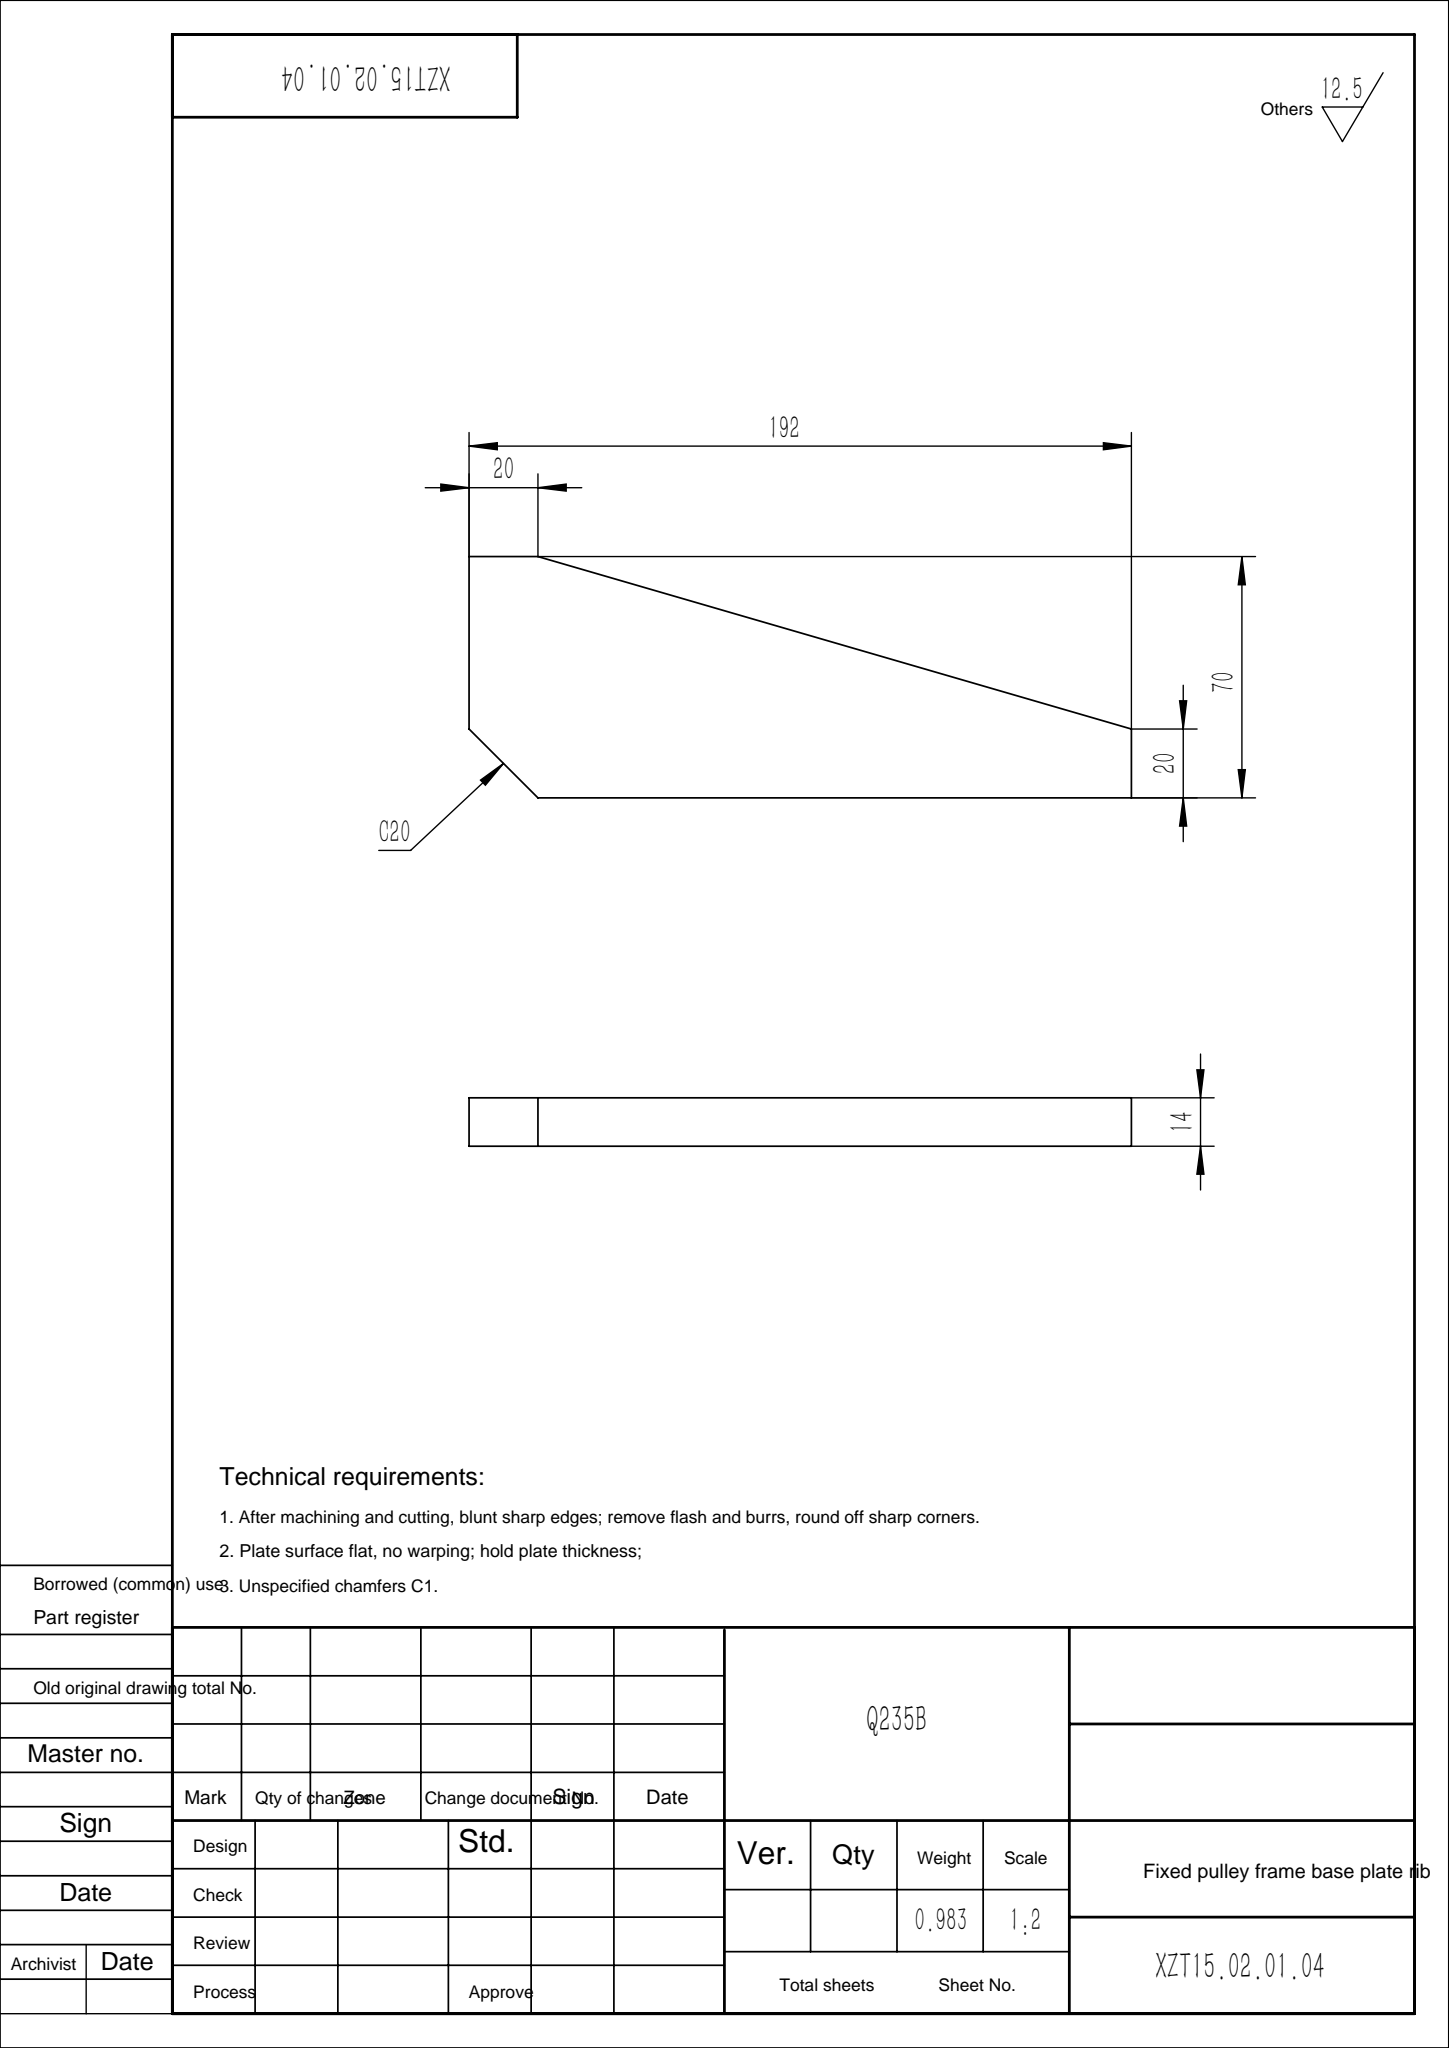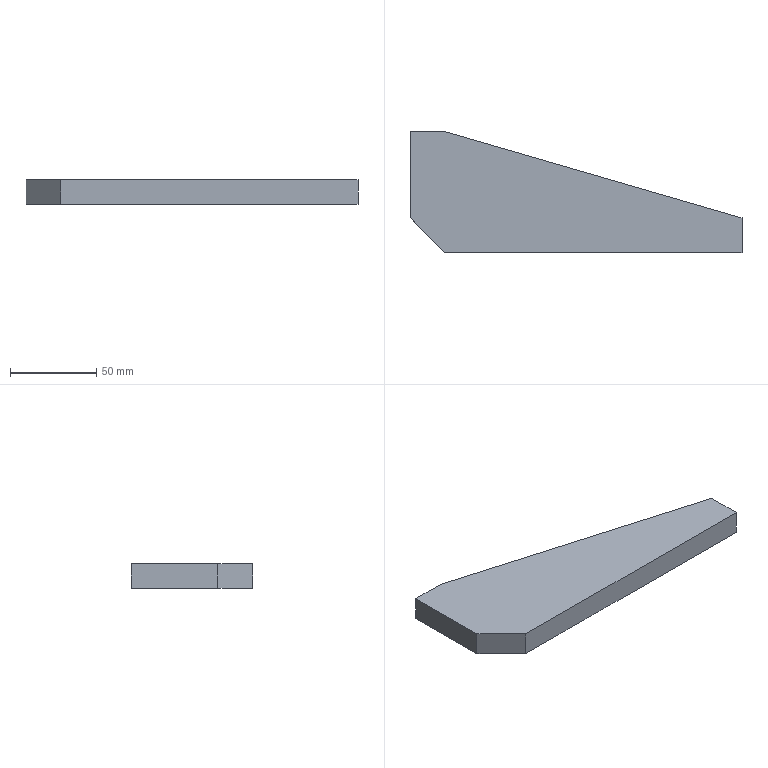Part | SolidWorks | features Chamfer 1, Extrusion 1 | 1 solid | 8 faces | box 192 x 70 x 14 mm | volume 125160 mm3 | plane 8
STEP:
#1=CARTESIAN_POINT('',(0.,70.,-7.));
#2=VERTEX_POINT('',#1);
#3=CARTESIAN_POINT('',(0.,20.,-7.));
#4=VERTEX_POINT('',#3);
#5=CARTESIAN_POINT('',(0.,70.,-7.));
#6=DIRECTION('',(0.,-1.,0.));
#7=VECTOR('',#6,1000.);
#8=LINE('',#5,#7);
#9=EDGE_CURVE('',#2,#4,#8,.T.);
#10=ORIENTED_EDGE('',*,*,#9,.T.);
#11=CARTESIAN_POINT('',(0.,20.,7.));
#12=VERTEX_POINT('',#11);
#13=CARTESIAN_POINT('',(0.,20.,7.));
#14=DIRECTION('',(0.,0.,1.));
#15=VECTOR('',#14,1000.);
#16=LINE('',#13,#15);
#17=EDGE_CURVE('',#4,#12,#16,.T.);
#18=ORIENTED_EDGE('',*,*,#17,.T.);
#19=CARTESIAN_POINT('',(0.,70.,7.));
#20=VERTEX_POINT('',#19);
#21=CARTESIAN_POINT('',(0.,70.,7.));
#22=DIRECTION('',(0.,-1.,0.));
#23=VECTOR('',#22,1000.);
#24=LINE('',#21,#23);
#25=EDGE_CURVE('',#20,#12,#24,.T.);
#26=ORIENTED_EDGE('',*,*,#25,.F.);
#27=CARTESIAN_POINT('',(0.,70.,7.));
#28=DIRECTION('',(0.,0.,-1.));
#29=VECTOR('',#28,1000.);
#30=LINE('',#27,#29);
#31=EDGE_CURVE('',#20,#2,#30,.T.);
#32=ORIENTED_EDGE('',*,*,#31,.T.);
#33=EDGE_LOOP('',(#10,#18,#26,#32));
#34=FACE_OUTER_BOUND('',#33,.T.);
#35=CARTESIAN_POINT('',(0.,70.,7.));
#36=DIRECTION('',(1.,0.,0.));
#37=DIRECTION('',(0.,1.,0.));
#38=AXIS2_PLACEMENT_3D('',#35,#36,#37);
#39=PLANE('',#38);
#40=ADVANCED_FACE('',(#34),#39,.F.);
#41=CARTESIAN_POINT('',(20.,0.,7.));
#42=VERTEX_POINT('',#41);
#43=CARTESIAN_POINT('',(192.,0.,7.));
#44=VERTEX_POINT('',#43);
#45=CARTESIAN_POINT('',(0.,0.,7.));
#46=DIRECTION('',(1.,0.,0.));
#47=VECTOR('',#46,1000.);
#48=LINE('',#45,#47);
#49=EDGE_CURVE('',#42,#44,#48,.T.);
#50=ORIENTED_EDGE('',*,*,#49,.F.);
#51=CARTESIAN_POINT('',(20.,0.,-7.));
#52=VERTEX_POINT('',#51);
#53=CARTESIAN_POINT('',(20.,0.,7.));
#54=DIRECTION('',(0.,0.,-1.));
#55=VECTOR('',#54,1000.);
#56=LINE('',#53,#55);
#57=EDGE_CURVE('',#42,#52,#56,.T.);
#58=ORIENTED_EDGE('',*,*,#57,.T.);
#59=CARTESIAN_POINT('',(192.,0.,-7.));
#60=VERTEX_POINT('',#59);
#61=CARTESIAN_POINT('',(0.,0.,-7.));
#62=DIRECTION('',(1.,0.,0.));
#63=VECTOR('',#62,1000.);
#64=LINE('',#61,#63);
#65=EDGE_CURVE('',#52,#60,#64,.T.);
#66=ORIENTED_EDGE('',*,*,#65,.T.);
#67=CARTESIAN_POINT('',(192.,0.,7.));
#68=DIRECTION('',(0.,0.,-1.));
#69=VECTOR('',#68,1000.);
#70=LINE('',#67,#69);
#71=EDGE_CURVE('',#44,#60,#70,.T.);
#72=ORIENTED_EDGE('',*,*,#71,.F.);
#73=EDGE_LOOP('',(#50,#58,#66,#72));
#74=FACE_OUTER_BOUND('',#73,.T.);
#75=CARTESIAN_POINT('',(0.,0.,7.));
#76=DIRECTION('',(0.,1.,0.));
#77=DIRECTION('',(0.,0.,1.));
#78=AXIS2_PLACEMENT_3D('',#75,#76,#77);
#79=PLANE('',#78);
#80=ADVANCED_FACE('',(#74),#79,.F.);
#81=CARTESIAN_POINT('',(192.,20.,-7.));
#82=VERTEX_POINT('',#81);
#83=CARTESIAN_POINT('',(192.,0.,-7.));
#84=DIRECTION('',(0.,1.,0.));
#85=VECTOR('',#84,1000.);
#86=LINE('',#83,#85);
#87=EDGE_CURVE('',#60,#82,#86,.T.);
#88=ORIENTED_EDGE('',*,*,#87,.T.);
#89=CARTESIAN_POINT('',(192.,20.,7.));
#90=VERTEX_POINT('',#89);
#91=CARTESIAN_POINT('',(192.,20.,7.));
#92=DIRECTION('',(0.,0.,-1.));
#93=VECTOR('',#92,1000.);
#94=LINE('',#91,#93);
#95=EDGE_CURVE('',#90,#82,#94,.T.);
#96=ORIENTED_EDGE('',*,*,#95,.F.);
#97=CARTESIAN_POINT('',(192.,0.,7.));
#98=DIRECTION('',(0.,1.,0.));
#99=VECTOR('',#98,1000.);
#100=LINE('',#97,#99);
#101=EDGE_CURVE('',#44,#90,#100,.T.);
#102=ORIENTED_EDGE('',*,*,#101,.F.);
#103=ORIENTED_EDGE('',*,*,#71,.T.);
#104=EDGE_LOOP('',(#88,#96,#102,#103));
#105=FACE_OUTER_BOUND('',#104,.T.);
#106=CARTESIAN_POINT('',(192.,0.,7.));
#107=DIRECTION('',(-1.,0.,0.));
#108=DIRECTION('',(0.,0.,1.));
#109=AXIS2_PLACEMENT_3D('',#106,#107,#108);
#110=PLANE('',#109);
#111=ADVANCED_FACE('',(#105),#110,.F.);
#112=CARTESIAN_POINT('',(20.,70.,-7.));
#113=VERTEX_POINT('',#112);
#114=CARTESIAN_POINT('',(192.,20.,-7.));
#115=DIRECTION('',(-0.9602,0.2791,0.));
#116=VECTOR('',#115,1000.);
#117=LINE('',#114,#116);
#118=EDGE_CURVE('',#82,#113,#117,.T.);
#119=ORIENTED_EDGE('',*,*,#118,.T.);
#120=CARTESIAN_POINT('',(20.,70.,7.));
#121=VERTEX_POINT('',#120);
#122=CARTESIAN_POINT('',(20.,70.,7.));
#123=DIRECTION('',(0.,0.,-1.));
#124=VECTOR('',#123,1000.);
#125=LINE('',#122,#124);
#126=EDGE_CURVE('',#121,#113,#125,.T.);
#127=ORIENTED_EDGE('',*,*,#126,.F.);
#128=CARTESIAN_POINT('',(192.,20.,7.));
#129=DIRECTION('',(-0.9602,0.2791,0.));
#130=VECTOR('',#129,1000.);
#131=LINE('',#128,#130);
#132=EDGE_CURVE('',#90,#121,#131,.T.);
#133=ORIENTED_EDGE('',*,*,#132,.F.);
#134=ORIENTED_EDGE('',*,*,#95,.T.);
#135=EDGE_LOOP('',(#119,#127,#133,#134));
#136=FACE_OUTER_BOUND('',#135,.T.);
#137=CARTESIAN_POINT('',(192.,20.,7.));
#138=DIRECTION('',(-0.2791,-0.9602,0.));
#139=DIRECTION('',(0.9602,-0.2791,0.));
#140=AXIS2_PLACEMENT_3D('',#137,#138,#139);
#141=PLANE('',#140);
#142=ADVANCED_FACE('',(#136),#141,.F.);
#143=CARTESIAN_POINT('',(20.,70.,-7.));
#144=DIRECTION('',(-1.,0.,0.));
#145=VECTOR('',#144,1000.);
#146=LINE('',#143,#145);
#147=EDGE_CURVE('',#113,#2,#146,.T.);
#148=ORIENTED_EDGE('',*,*,#147,.T.);
#149=ORIENTED_EDGE('',*,*,#31,.F.);
#150=CARTESIAN_POINT('',(20.,70.,7.));
#151=DIRECTION('',(-1.,0.,0.));
#152=VECTOR('',#151,1000.);
#153=LINE('',#150,#152);
#154=EDGE_CURVE('',#121,#20,#153,.T.);
#155=ORIENTED_EDGE('',*,*,#154,.F.);
#156=ORIENTED_EDGE('',*,*,#126,.T.);
#157=EDGE_LOOP('',(#148,#149,#155,#156));
#158=FACE_OUTER_BOUND('',#157,.T.);
#159=CARTESIAN_POINT('',(20.,70.,7.));
#160=DIRECTION('',(0.,-1.,0.));
#161=DIRECTION('',(0.,0.,-1.));
#162=AXIS2_PLACEMENT_3D('',#159,#160,#161);
#163=PLANE('',#162);
#164=ADVANCED_FACE('',(#158),#163,.F.);
#165=ORIENTED_EDGE('',*,*,#25,.T.);
#166=CARTESIAN_POINT('',(10.,10.,7.));
#167=DIRECTION('',(0.7071,-0.7071,0.));
#168=VECTOR('',#167,1000.);
#169=LINE('',#166,#168);
#170=EDGE_CURVE('',#12,#42,#169,.T.);
#171=ORIENTED_EDGE('',*,*,#170,.T.);
#172=ORIENTED_EDGE('',*,*,#49,.T.);
#173=ORIENTED_EDGE('',*,*,#101,.T.);
#174=ORIENTED_EDGE('',*,*,#132,.T.);
#175=ORIENTED_EDGE('',*,*,#154,.T.);
#176=EDGE_LOOP('',(#165,#171,#172,#173,#174,#175));
#177=FACE_OUTER_BOUND('',#176,.T.);
#178=CARTESIAN_POINT('',(0.,0.,7.));
#179=DIRECTION('',(0.,0.,1.));
#180=DIRECTION('',(1.,0.,0.));
#181=AXIS2_PLACEMENT_3D('',#178,#179,#180);
#182=PLANE('',#181);
#183=ADVANCED_FACE('',(#177),#182,.T.);
#184=ORIENTED_EDGE('',*,*,#65,.F.);
#185=CARTESIAN_POINT('',(20.,0.,-7.));
#186=DIRECTION('',(-0.7071,0.7071,0.));
#187=VECTOR('',#186,1000.);
#188=LINE('',#185,#187);
#189=EDGE_CURVE('',#52,#4,#188,.T.);
#190=ORIENTED_EDGE('',*,*,#189,.T.);
#191=ORIENTED_EDGE('',*,*,#9,.F.);
#192=ORIENTED_EDGE('',*,*,#147,.F.);
#193=ORIENTED_EDGE('',*,*,#118,.F.);
#194=ORIENTED_EDGE('',*,*,#87,.F.);
#195=EDGE_LOOP('',(#184,#190,#191,#192,#193,#194));
#196=FACE_OUTER_BOUND('',#195,.T.);
#197=CARTESIAN_POINT('',(0.,0.,-7.));
#198=DIRECTION('',(0.,0.,1.));
#199=DIRECTION('',(1.,0.,0.));
#200=AXIS2_PLACEMENT_3D('',#197,#198,#199);
#201=PLANE('',#200);
#202=ADVANCED_FACE('',(#196),#201,.F.);
#203=ORIENTED_EDGE('',*,*,#170,.F.);
#204=ORIENTED_EDGE('',*,*,#17,.F.);
#205=ORIENTED_EDGE('',*,*,#189,.F.);
#206=ORIENTED_EDGE('',*,*,#57,.F.);
#207=EDGE_LOOP('',(#203,#204,#205,#206));
#208=FACE_OUTER_BOUND('',#207,.T.);
#209=CARTESIAN_POINT('',(20.,0.,7.));
#210=DIRECTION('',(0.7071,0.7071,0.));
#211=DIRECTION('',(0.,0.,-1.));
#212=AXIS2_PLACEMENT_3D('',#209,#210,#211);
#213=PLANE('',#212);
#214=ADVANCED_FACE('',(#208),#213,.F.);
#215=CLOSED_SHELL('',(#40,#80,#111,#142,#164,#183,#202,#214));
#216=MANIFOLD_SOLID_BREP('',#215);
#217=CARTESIAN_POINT('',(0.,0.,0.));
#218=DIRECTION('',(0.,0.,1.));
#219=DIRECTION('',(1.,0.,0.));
#220=AXIS2_PLACEMENT_3D('',#217,#218,#219);
#221=(LENGTH_UNIT()NAMED_UNIT(*)SI_UNIT(.MILLI.,.METRE.));
#222=UNCERTAINTY_MEASURE_WITH_UNIT(LENGTH_MEASURE(0.00001),#221,'','');
#223=(NAMED_UNIT(*)PLANE_ANGLE_UNIT()SI_UNIT($,.RADIAN.));
#224=(NAMED_UNIT(*)SI_UNIT($,.STERADIAN.)SOLID_ANGLE_UNIT());
#225=(GEOMETRIC_REPRESENTATION_CONTEXT(3)GLOBAL_UNCERTAINTY_ASSIGNED_CONTEXT((#222))GLOBAL_UNIT_ASSIGNED_CONTEXT((#221,#223,#224))REPRESENTATION_CONTEXT('',''));
#226=ADVANCED_BREP_SHAPE_REPRESENTATION('',(#216,#220),#225);